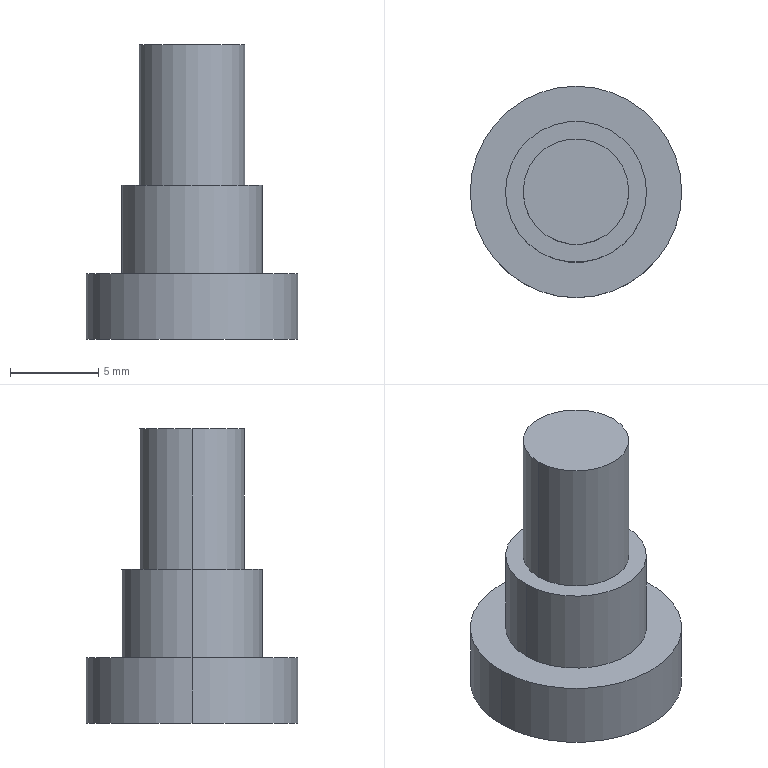Part | SolidWorks | features ICE 2, Extrusion 1, MoveCopyBody 1 | 1 solid | 10 faces | box 12 x 12 x 16.74 mm | volume 900.506 mm3 | cylinder 6 | plane 4 | commonest cylinder face diameters 6 x2 8 x2 12 x2
STEP:
#1=CARTESIAN_POINT('',(3.,0.,16.74));
#2=VERTEX_POINT('',#1);
#3=CARTESIAN_POINT('',(-3.,0.,16.74));
#4=VERTEX_POINT('',#3);
#5=CARTESIAN_POINT('',(0.,0.,16.74));
#6=DIRECTION('',(0.,0.,1.));
#7=DIRECTION('',(1.,0.,0.));
#8=AXIS2_PLACEMENT_3D('',#5,#6,#7);
#9=CIRCLE('',#8,3.);
#10=EDGE_CURVE('',#2,#4,#9,.T.);
#11=ORIENTED_EDGE('',*,*,#10,.F.);
#12=CARTESIAN_POINT('',(3.,0.,8.74));
#13=VERTEX_POINT('',#12);
#14=CARTESIAN_POINT('',(3.,0.,16.74));
#15=DIRECTION('',(0.,0.,-1.));
#16=VECTOR('',#15,1000.);
#17=LINE('',#14,#16);
#18=EDGE_CURVE('',#2,#13,#17,.T.);
#19=ORIENTED_EDGE('',*,*,#18,.T.);
#20=CARTESIAN_POINT('',(-3.,0.,8.74));
#21=VERTEX_POINT('',#20);
#22=CARTESIAN_POINT('',(0.,0.,8.74));
#23=DIRECTION('',(0.,0.,1.));
#24=DIRECTION('',(1.,0.,0.));
#25=AXIS2_PLACEMENT_3D('',#22,#23,#24);
#26=CIRCLE('',#25,3.);
#27=EDGE_CURVE('',#13,#21,#26,.T.);
#28=ORIENTED_EDGE('',*,*,#27,.T.);
#29=CARTESIAN_POINT('',(-3.,0.,16.74));
#30=DIRECTION('',(0.,0.,-1.));
#31=VECTOR('',#30,1000.);
#32=LINE('',#29,#31);
#33=EDGE_CURVE('',#4,#21,#32,.T.);
#34=ORIENTED_EDGE('',*,*,#33,.F.);
#35=EDGE_LOOP('',(#11,#19,#28,#34));
#36=FACE_OUTER_BOUND('',#35,.T.);
#37=CARTESIAN_POINT('',(0.,0.,16.74));
#38=DIRECTION('',(0.,0.,-1.));
#39=DIRECTION('',(-1.,0.,0.));
#40=AXIS2_PLACEMENT_3D('',#37,#38,#39);
#41=CYLINDRICAL_SURFACE('',#40,3.);
#42=ADVANCED_FACE('',(#36),#41,.T.);
#43=CARTESIAN_POINT('',(4.,0.,8.74));
#44=VERTEX_POINT('',#43);
#45=CARTESIAN_POINT('',(-4.,0.,8.74));
#46=VERTEX_POINT('',#45);
#47=CARTESIAN_POINT('',(0.,0.,8.74));
#48=DIRECTION('',(0.,0.,1.));
#49=DIRECTION('',(1.,0.,0.));
#50=AXIS2_PLACEMENT_3D('',#47,#48,#49);
#51=CIRCLE('',#50,4.);
#52=EDGE_CURVE('',#44,#46,#51,.T.);
#53=ORIENTED_EDGE('',*,*,#52,.F.);
#54=CARTESIAN_POINT('',(4.,0.,3.74));
#55=VERTEX_POINT('',#54);
#56=CARTESIAN_POINT('',(4.,0.,8.74));
#57=DIRECTION('',(0.,0.,-1.));
#58=VECTOR('',#57,1000.);
#59=LINE('',#56,#58);
#60=EDGE_CURVE('',#44,#55,#59,.T.);
#61=ORIENTED_EDGE('',*,*,#60,.T.);
#62=CARTESIAN_POINT('',(-4.,0.,3.74));
#63=VERTEX_POINT('',#62);
#64=CARTESIAN_POINT('',(0.,0.,3.74));
#65=DIRECTION('',(0.,0.,1.));
#66=DIRECTION('',(1.,0.,0.));
#67=AXIS2_PLACEMENT_3D('',#64,#65,#66);
#68=CIRCLE('',#67,4.);
#69=EDGE_CURVE('',#55,#63,#68,.T.);
#70=ORIENTED_EDGE('',*,*,#69,.T.);
#71=CARTESIAN_POINT('',(-4.,0.,8.74));
#72=DIRECTION('',(0.,0.,-1.));
#73=VECTOR('',#72,1000.);
#74=LINE('',#71,#73);
#75=EDGE_CURVE('',#46,#63,#74,.T.);
#76=ORIENTED_EDGE('',*,*,#75,.F.);
#77=EDGE_LOOP('',(#53,#61,#70,#76));
#78=FACE_OUTER_BOUND('',#77,.T.);
#79=CARTESIAN_POINT('',(0.,0.,8.74));
#80=DIRECTION('',(0.,0.,-1.));
#81=DIRECTION('',(-1.,0.,0.));
#82=AXIS2_PLACEMENT_3D('',#79,#80,#81);
#83=CYLINDRICAL_SURFACE('',#82,4.);
#84=ADVANCED_FACE('',(#78),#83,.T.);
#85=CARTESIAN_POINT('',(6.,0.,3.74));
#86=VERTEX_POINT('',#85);
#87=CARTESIAN_POINT('',(-6.,0.,3.74));
#88=VERTEX_POINT('',#87);
#89=CARTESIAN_POINT('',(0.,0.,3.74));
#90=DIRECTION('',(0.,0.,1.));
#91=DIRECTION('',(1.,0.,0.));
#92=AXIS2_PLACEMENT_3D('',#89,#90,#91);
#93=CIRCLE('',#92,6.);
#94=EDGE_CURVE('',#86,#88,#93,.T.);
#95=ORIENTED_EDGE('',*,*,#94,.F.);
#96=CARTESIAN_POINT('',(6.,0.,0.));
#97=VERTEX_POINT('',#96);
#98=CARTESIAN_POINT('',(6.,0.,3.74));
#99=DIRECTION('',(0.,0.,-1.));
#100=VECTOR('',#99,1000.);
#101=LINE('',#98,#100);
#102=EDGE_CURVE('',#86,#97,#101,.T.);
#103=ORIENTED_EDGE('',*,*,#102,.T.);
#104=CARTESIAN_POINT('',(-6.,0.,0.));
#105=VERTEX_POINT('',#104);
#106=CARTESIAN_POINT('',(0.,0.,0.));
#107=DIRECTION('',(0.,0.,1.));
#108=DIRECTION('',(1.,0.,0.));
#109=AXIS2_PLACEMENT_3D('',#106,#107,#108);
#110=CIRCLE('',#109,6.);
#111=EDGE_CURVE('',#97,#105,#110,.T.);
#112=ORIENTED_EDGE('',*,*,#111,.T.);
#113=CARTESIAN_POINT('',(-6.,0.,3.74));
#114=DIRECTION('',(0.,0.,-1.));
#115=VECTOR('',#114,1000.);
#116=LINE('',#113,#115);
#117=EDGE_CURVE('',#88,#105,#116,.T.);
#118=ORIENTED_EDGE('',*,*,#117,.F.);
#119=EDGE_LOOP('',(#95,#103,#112,#118));
#120=FACE_OUTER_BOUND('',#119,.T.);
#121=CARTESIAN_POINT('',(0.,0.,3.74));
#122=DIRECTION('',(0.,0.,-1.));
#123=DIRECTION('',(-1.,0.,0.));
#124=AXIS2_PLACEMENT_3D('',#121,#122,#123);
#125=CYLINDRICAL_SURFACE('',#124,6.);
#126=ADVANCED_FACE('',(#120),#125,.T.);
#127=ORIENTED_EDGE('',*,*,#102,.F.);
#128=CARTESIAN_POINT('',(0.,0.,3.74));
#129=DIRECTION('',(0.,0.,1.));
#130=DIRECTION('',(1.,0.,0.));
#131=AXIS2_PLACEMENT_3D('',#128,#129,#130);
#132=CIRCLE('',#131,6.);
#133=EDGE_CURVE('',#88,#86,#132,.T.);
#134=ORIENTED_EDGE('',*,*,#133,.F.);
#135=ORIENTED_EDGE('',*,*,#117,.T.);
#136=CARTESIAN_POINT('',(0.,0.,0.));
#137=DIRECTION('',(0.,0.,1.));
#138=DIRECTION('',(1.,0.,0.));
#139=AXIS2_PLACEMENT_3D('',#136,#137,#138);
#140=CIRCLE('',#139,6.);
#141=EDGE_CURVE('',#105,#97,#140,.T.);
#142=ORIENTED_EDGE('',*,*,#141,.T.);
#143=EDGE_LOOP('',(#127,#134,#135,#142));
#144=FACE_OUTER_BOUND('',#143,.T.);
#145=CARTESIAN_POINT('',(0.,0.,3.74));
#146=DIRECTION('',(0.,0.,-1.));
#147=DIRECTION('',(-1.,0.,0.));
#148=AXIS2_PLACEMENT_3D('',#145,#146,#147);
#149=CYLINDRICAL_SURFACE('',#148,6.);
#150=ADVANCED_FACE('',(#144),#149,.T.);
#151=CARTESIAN_POINT('',(0.,0.,3.74));
#152=DIRECTION('',(0.,0.,1.));
#153=DIRECTION('',(1.,0.,0.));
#154=AXIS2_PLACEMENT_3D('',#151,#152,#153);
#155=CIRCLE('',#154,4.);
#156=EDGE_CURVE('',#63,#55,#155,.T.);
#157=ORIENTED_EDGE('',*,*,#156,.F.);
#158=ORIENTED_EDGE('',*,*,#69,.F.);
#159=EDGE_LOOP('',(#157,#158));
#160=FACE_BOUND('',#159,.T.);
#161=ORIENTED_EDGE('',*,*,#133,.T.);
#162=ORIENTED_EDGE('',*,*,#94,.T.);
#163=EDGE_LOOP('',(#161,#162));
#164=FACE_OUTER_BOUND('',#163,.T.);
#165=CARTESIAN_POINT('',(0.,0.,3.74));
#166=DIRECTION('',(0.,0.,1.));
#167=DIRECTION('',(1.,0.,0.));
#168=AXIS2_PLACEMENT_3D('',#165,#166,#167);
#169=PLANE('',#168);
#170=ADVANCED_FACE('',(#160,#164),#169,.T.);
#171=ORIENTED_EDGE('',*,*,#141,.F.);
#172=ORIENTED_EDGE('',*,*,#111,.F.);
#173=EDGE_LOOP('',(#171,#172));
#174=FACE_OUTER_BOUND('',#173,.T.);
#175=CARTESIAN_POINT('',(0.,0.,0.));
#176=DIRECTION('',(0.,0.,1.));
#177=DIRECTION('',(1.,0.,0.));
#178=AXIS2_PLACEMENT_3D('',#175,#176,#177);
#179=PLANE('',#178);
#180=ADVANCED_FACE('',(#174),#179,.F.);
#181=ORIENTED_EDGE('',*,*,#60,.F.);
#182=CARTESIAN_POINT('',(0.,0.,8.74));
#183=DIRECTION('',(0.,0.,1.));
#184=DIRECTION('',(1.,0.,0.));
#185=AXIS2_PLACEMENT_3D('',#182,#183,#184);
#186=CIRCLE('',#185,4.);
#187=EDGE_CURVE('',#46,#44,#186,.T.);
#188=ORIENTED_EDGE('',*,*,#187,.F.);
#189=ORIENTED_EDGE('',*,*,#75,.T.);
#190=ORIENTED_EDGE('',*,*,#156,.T.);
#191=EDGE_LOOP('',(#181,#188,#189,#190));
#192=FACE_OUTER_BOUND('',#191,.T.);
#193=CARTESIAN_POINT('',(0.,0.,8.74));
#194=DIRECTION('',(0.,0.,-1.));
#195=DIRECTION('',(-1.,0.,0.));
#196=AXIS2_PLACEMENT_3D('',#193,#194,#195);
#197=CYLINDRICAL_SURFACE('',#196,4.);
#198=ADVANCED_FACE('',(#192),#197,.T.);
#199=CARTESIAN_POINT('',(0.,0.,8.74));
#200=DIRECTION('',(0.,0.,1.));
#201=DIRECTION('',(1.,0.,0.));
#202=AXIS2_PLACEMENT_3D('',#199,#200,#201);
#203=CIRCLE('',#202,3.);
#204=EDGE_CURVE('',#21,#13,#203,.T.);
#205=ORIENTED_EDGE('',*,*,#204,.F.);
#206=ORIENTED_EDGE('',*,*,#27,.F.);
#207=EDGE_LOOP('',(#205,#206));
#208=FACE_BOUND('',#207,.T.);
#209=ORIENTED_EDGE('',*,*,#187,.T.);
#210=ORIENTED_EDGE('',*,*,#52,.T.);
#211=EDGE_LOOP('',(#209,#210));
#212=FACE_OUTER_BOUND('',#211,.T.);
#213=CARTESIAN_POINT('',(0.,0.,8.74));
#214=DIRECTION('',(0.,0.,1.));
#215=DIRECTION('',(1.,0.,0.));
#216=AXIS2_PLACEMENT_3D('',#213,#214,#215);
#217=PLANE('',#216);
#218=ADVANCED_FACE('',(#208,#212),#217,.T.);
#219=ORIENTED_EDGE('',*,*,#18,.F.);
#220=CARTESIAN_POINT('',(0.,0.,16.74));
#221=DIRECTION('',(0.,0.,1.));
#222=DIRECTION('',(1.,0.,0.));
#223=AXIS2_PLACEMENT_3D('',#220,#221,#222);
#224=CIRCLE('',#223,3.);
#225=EDGE_CURVE('',#4,#2,#224,.T.);
#226=ORIENTED_EDGE('',*,*,#225,.F.);
#227=ORIENTED_EDGE('',*,*,#33,.T.);
#228=ORIENTED_EDGE('',*,*,#204,.T.);
#229=EDGE_LOOP('',(#219,#226,#227,#228));
#230=FACE_OUTER_BOUND('',#229,.T.);
#231=CARTESIAN_POINT('',(0.,0.,16.74));
#232=DIRECTION('',(0.,0.,-1.));
#233=DIRECTION('',(-1.,0.,0.));
#234=AXIS2_PLACEMENT_3D('',#231,#232,#233);
#235=CYLINDRICAL_SURFACE('',#234,3.);
#236=ADVANCED_FACE('',(#230),#235,.T.);
#237=ORIENTED_EDGE('',*,*,#225,.T.);
#238=ORIENTED_EDGE('',*,*,#10,.T.);
#239=EDGE_LOOP('',(#237,#238));
#240=FACE_OUTER_BOUND('',#239,.T.);
#241=CARTESIAN_POINT('',(0.,0.,16.74));
#242=DIRECTION('',(0.,0.,1.));
#243=DIRECTION('',(1.,0.,0.));
#244=AXIS2_PLACEMENT_3D('',#241,#242,#243);
#245=PLANE('',#244);
#246=ADVANCED_FACE('',(#240),#245,.T.);
#247=CLOSED_SHELL('',(#42,#84,#126,#150,#170,#180,#198,#218,#236,#246));
#248=MANIFOLD_SOLID_BREP('',#247);
#249=CARTESIAN_POINT('',(0.,0.,0.));
#250=DIRECTION('',(0.,0.,1.));
#251=DIRECTION('',(1.,0.,0.));
#252=AXIS2_PLACEMENT_3D('',#249,#250,#251);
#253=(LENGTH_UNIT()NAMED_UNIT(*)SI_UNIT(.MILLI.,.METRE.));
#254=UNCERTAINTY_MEASURE_WITH_UNIT(LENGTH_MEASURE(0.00001),#253,'','');
#255=(NAMED_UNIT(*)PLANE_ANGLE_UNIT()SI_UNIT($,.RADIAN.));
#256=(NAMED_UNIT(*)SI_UNIT($,.STERADIAN.)SOLID_ANGLE_UNIT());
#257=(GEOMETRIC_REPRESENTATION_CONTEXT(3)GLOBAL_UNCERTAINTY_ASSIGNED_CONTEXT((#254))GLOBAL_UNIT_ASSIGNED_CONTEXT((#253,#255,#256))REPRESENTATION_CONTEXT('',''));
#258=ADVANCED_BREP_SHAPE_REPRESENTATION('',(#248,#252),#257);